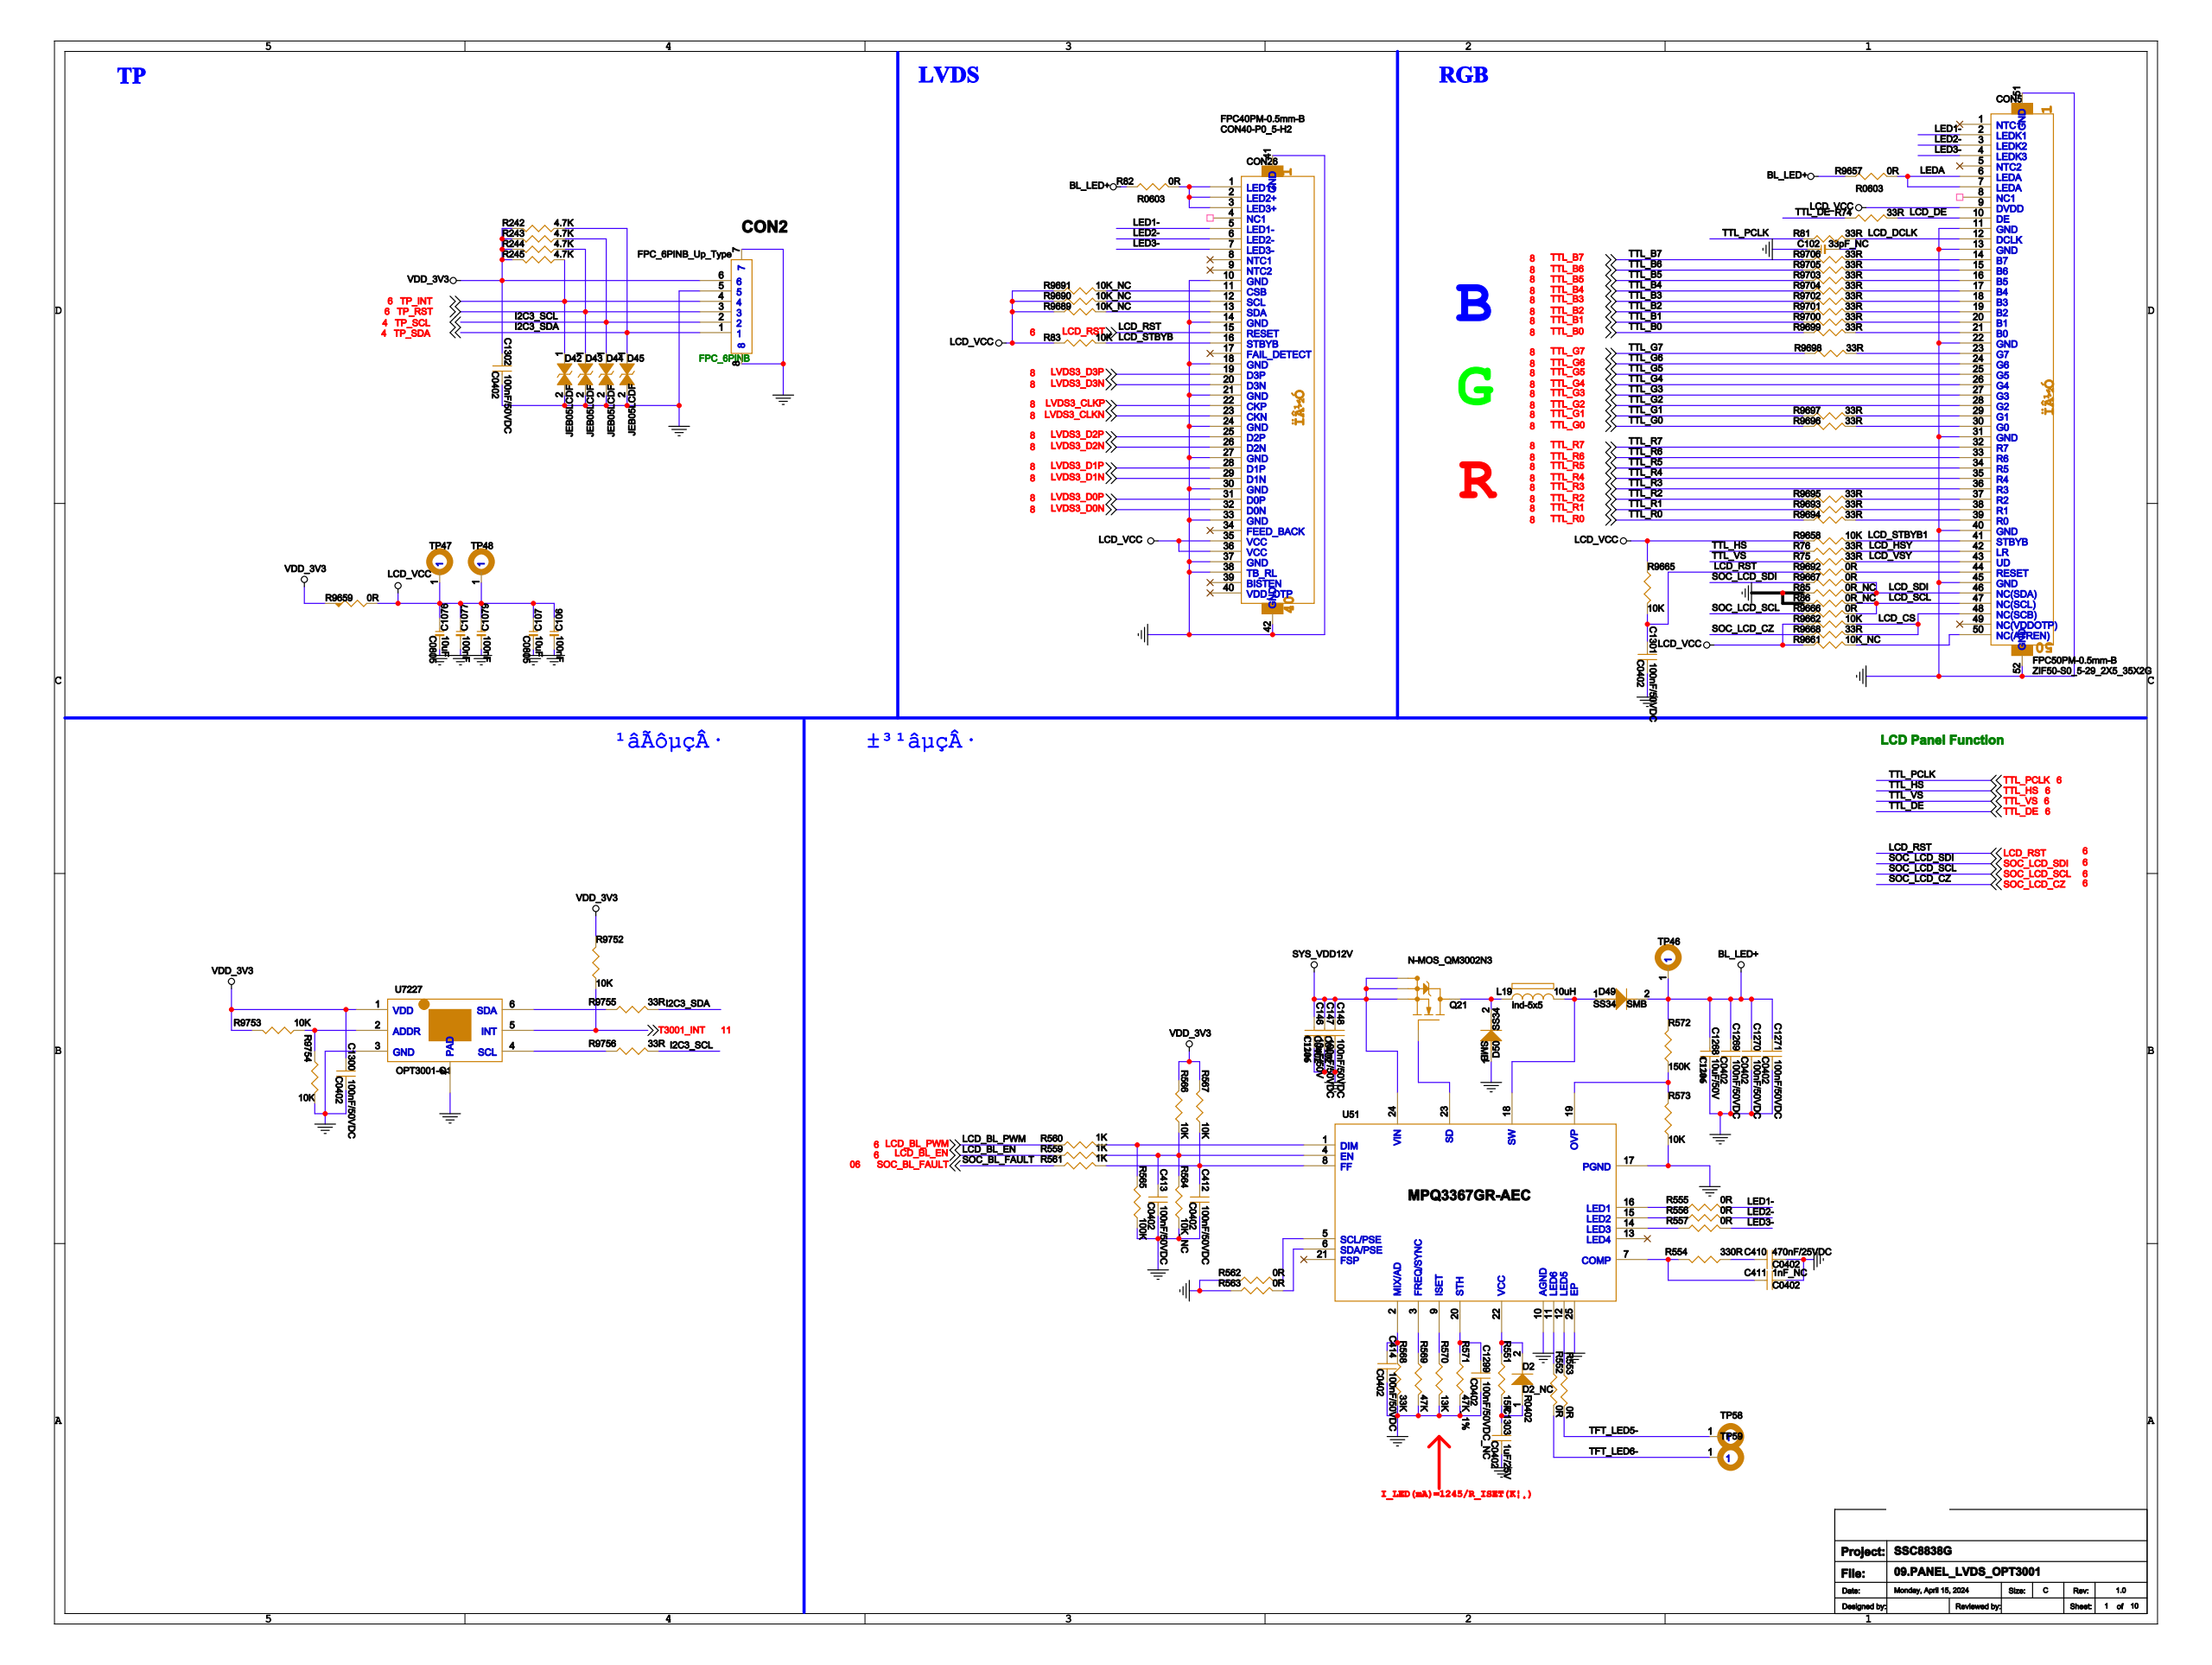Circuit board | Cadence Allegro | 958 parts | 601 nets | one sheet of the schematic
Parts on this sheet (reference | value | footprint):
C102 | 33pF_NC | C0402
C106 | 100nF | C0402
C107 | 10uF | C0805
C146 | 10uF/50V | C1206
C147 | 100nF/50VDC | C0402
C148 | 100nF/50VDC | C0402
C410 | 470nF/25VDC | C0402
C411 | 1nF_NC | C0402
C412 | 100nF/50VDC | C0402
C413 | 100nF/50VDC | C0402
C414 | 100nF/50VDC | C0402
C1076 | 10uF | C0805
C1077 | 100nF | C0402
C1079 | 100nF | C0402
C1268 | 10uF/50V | C1206
C1269 | 100nF/50VDC | C0402
C1270 | 100nF/50VDC | C0402
C1271 | 100nF/50VDC | C0402
C1299 | 100nF/50VDC_NC | C0402
C1300 | 100nF/50VDC | C0402
C1301 | 100nF/50VDC | C0402
C1302 | 100nF/50VDC | C0402
C1303 | 1uF/25V | C0402
CON2 | FPC_6PINB_Up_Type | FPC_6PINB
CON5 | FPC50PM-0.5mm-B | ZIF50-S0_5-29_2X5_35X2G
CON26 | FPC40PM-0.5mm-B | CON40-P0_5-H2
D2 | D2_NC | R0402
D49 | SS34 | SMB
D50 | SS34 | SMB
L19 | 10uH | IND-5X5
Q21 | N-MOS_QM3002N3 | N_MOS_QM3002N3
R74 | 33R | R0402
R75 | 33R | R0402
R76 | 33R | R0402
R81 | 33R | R0402
R82 | 0R | R0603
R83 | 10K | R0402
R85 | 0R_NC | R0402
R86 | 0R_NC | R0402
R242 | 4.7K | R0402
R243 | 4.7K | R0402
R244 | 4.7K | R0402
R245 | 4.7K | R0402
R551 | 15R | R0603
R552 | 0R | R0603
R553 | 0R | R0603
R554 | 330R | R0603
R555 | 0R | R0603
R556 | 0R | R0603
R557 | 0R | R0603
R559 | 1K | R0603
R560 | 1K | R0603
R561 | 1K | R0603
R562 | 0R | R0603
R563 | 0R | R0603
R564 | 10K_NC | R0603
R565 | 100K | R0603
R566 | 10K | R0603
R567 | 10K | R0603
R568 | 33K | R0603
R569 | 47K | R0603
R570 | 13K | R0603
R571 | 47K_1% | R0603
R572 | 150K | R0603
R573 | 10K | R0603
R9657 | 0R | R0603
R9658 | 10K | R0402
R9659 | 0R | R0402
R9661 | 10K_NC | R0402
R9662 | 10K | R0402
R9665 | 10K | R0402
R9666 | 0R | R0402
R9667 | 0R | R0402
R9668 | 33R | R0402
R9689 | 10K_NC | R0402
R9690 | 10K_NC | R0402
R9691 | 10K_NC | R0402
R9692 | 0R | R0402
R9693 | 33R | R0402
R9694 | 33R | R0402
R9695 | 33R | R0402
R9696 | 33R | R0402
R9697 | 33R | R0402
R9698 | 33R | R0402
R9699 | 33R | R0402
R9700 | 33R | R0402
R9701 | 33R | R0402
R9702 | 33R | R0402
R9703 | 33R | R0402
R9704 | 33R | R0402
R9705 | 33R | R0402
R9706 | 33R | R0402
R9752 | 10K | R0402
R9753 | 10K | R0402
R9755 | 33R | R0402
R9756 | 33R | R0402
TP46 | HOLE | TP_0R50
TP47 | HOLE | TP_0R50
TP48 | HOLE | TP_0R50
TP58 | HOLE | TP_0R50
TP59 | HOLE | TP_0R50
U51 | MPQ3367GR-AEC | QFN24-0_5-4X4X1T
U7227 | OPT3001-Q1 | DFN6-0_65-2X2X0_75T
Nets of these parts (net: part-pin ...):
GND: C102-1 C106-2 C107-2 C146-1 C147-2 C148-2 C410-2 C411-2 C412-2 C413-2 C414-2 C1076-2 C1077-2 C1079-2 C1268-1 C1269-2 C1270-2 C1271-2 C1299-2 C1300-2 C1301-2 C1302-2 C1303-2 CON2-5 CON2-7 CON2-8 D50-1 R85-1 R86-1 R562-2 R563-2 R564-2 R565-2 R568-1 R569-1 R570-1 R571-1 R573-2 U7227-3 U7227-7 CON5-11 CON5-13 CON5-22 CON5-31 CON5-40 CON5-45 CON5-51 CON5-52 CON26-10 CON26-14 CON26-18 CON26-21 CON26-24 CON26-27 CON26-30 CON26-33 CON26-37 CON26-38 CON26-41 CON26-42 U51-10 U51-17 U51-25
LCD_VCC: C106-1 C107-1 C1076-1 C1077-1 C1079-1 R83-1 R9658-1 R9659-2 R9661-1 R9662-1 R9665-1 R9689-1 R9690-1 R9691-1 TP47-1 TP48-1 CON5-9 CON26-35 CON26-36
SYS_VDD12V: C146-2 C147-1 C148-1 Q21-S1 Q21-S2 Q21-S3 U51-24
3V3_NORMAL: C1300-1 C1302-1 CON2-6 R242-1 R243-1 R244-1 R245-1 R566-1 R567-1 R9659-1 R9752-1 R9753-1 U7227-1
LCD_DCLK: C102-2 R81-2 CON5-12
BL_LED+: C1268-2 C1269-1 C1270-1 C1271-1 D49-2 R82-1 R572-1 R9657-1 TP46-1
LCD_RST: C1301-1 R9665-2 R9692-1 CON26-15
N21133766: C412-1 R561-1 R567-2 U51-8
N21133662: C413-1 R559-1 R564-1 R566-2 U51-4
N21140205: C414-1 R568-2 U51-2
N21143793: C1299-1 R571-2 U51-20
N21127354: C1303-1 D2-1 R551-1
N21129488: C410-1 R554-2
N21129474: C411-1 R554-1 U51-7
LVDS3_CLKP: CON26-22
LVDS3_CLKN: CON26-23
LVDS3_D0P: CON26-31
LVDS3_D0N: CON26-32
LVDS3_D1P: CON26-28
LVDS3_D1N: CON26-29
LVDS3_D2P: CON26-25
LVDS3_D2N: CON26-26
LVDS3_D3P: CON26-19
LVDS3_D3N: CON26-20
TP_SDA: CON2-1 R242-2 R9755-1
TP_SCL: CON2-2 R243-2 R9756-1
TP_RST: CON2-3 R244-2
TP_INT: CON2-4 R245-2
N21754242: R9691-2 CON26-11
N21313903: R82-2 CON26-1 CON26-2 CON26-3
LED1-: R555-1 CON5-2 CON26-5
LED2-: R556-1 CON5-3 CON26-6
LED3-: R557-1 CON5-4 CON26-7
N21754249: R9690-2 CON26-12
N21754525: R9689-2 CON26-13
LCD_STBYB: R83-2 CON26-16
N21343553: R9699-2 CON5-21
N21343427: R9700-2 CON5-20
N21343424: R9701-2 CON5-19
N21343421: R9702-2 CON5-18
N21343649: R9704-2 CON5-17
N21343652: R9703-2 CON5-16
N21343646: R9705-2 CON5-15
N21343643: R9706-2 CON5-14
LCD_DE: R74-2 CON5-10
N21343330: R9696-2 CON5-30
N21343333: R9697-2 CON5-29
TTL_G2: CON5-28
TTL_G3: CON5-27
TTL_G4: CON5-26
TTL_G5: CON5-25
TTL_G6: CON5-24
N21343369: R9698-2 CON5-23
LEDA: R9657-2 CON5-6 CON5-7
LCD_HSY: R76-2 CON5-42
N21325267: R9661-2 CON5-50
LCD_CS: R9662-2 R9668-2 CON5-48
LCD_SCL: R86-2 R9666-2 CON5-47
LCD_SDI: R85-2 R9667-2 CON5-46
N21343141: R9694-2 CON5-39
N21343138: R9693-2 CON5-38
N21343189: R9695-2 CON5-37
TTL_R3: CON5-36
TTL_R4: CON5-35
TTL_R5: CON5-34
TTL_R6: CON5-33
TTL_R7: CON5-32
N21339485: R9692-2 CON5-44
LCD_STBYB1: R9658-2 CON5-41
LCD_VSY: R75-2 CON5-43
N21127326: D2-2 R551-2 U51-22
N21145386: D49-1 L19-2 U51-18
N21146254: D50-2 L19-1 Q21-D1
N21146233: Q21-G U51-23
TFT_LED6-: R552-1 TP59-1
N21128932: R552-2 U51-11
TFT_LED5-: R553-1 TP58-1
N21128939: R553-2 U51-12
N21132365: R555-2 U51-16
N21132385: R556-2 U51-15
N21132405: R557-2 U51-14
N21136897: R562-1 U51-5
N21134064: R563-1 U51-6
LCD_BL_EN: R559-2
N21133726: R560-1 R565-1 U51-1
LCD_BL_PWM: R560-2
SOC_BL_FAULT: R561-2
N21144334: R572-2 R573-1 U51-19
N21141600: R569-2 U51-3
N21143041: R570-2 U51-9
TTL_DE: R74-1
TTL_VS: R75-1
TTL_HS: R76-1
TTL_PCLK: R81-1
SOC_LCD_CZ: R9668-1
TTL_R1: R9693-1
TTL_R0: R9694-1
TTL_R2: R9695-1
TTL_G0: R9696-1
TTL_G1: R9697-1
TTL_G7: R9698-1
TTL_B0: R9699-1
TTL_B1: R9700-1
TTL_B2: R9701-1
TTL_B3: R9702-1
TTL_B5: R9703-1
TTL_B4: R9704-1
TTL_B6: R9705-1
TTL_B7: R9706-1
SOC_LCD_SCL: R9666-1
SOC_LCD_SDI: R9667-1
T3001_INT: R9752-2 U7227-5
N21445879: R9753-2 U7227-2
N21444465: R9755-2 U7227-6
N21444495: R9756-2 U7227-4